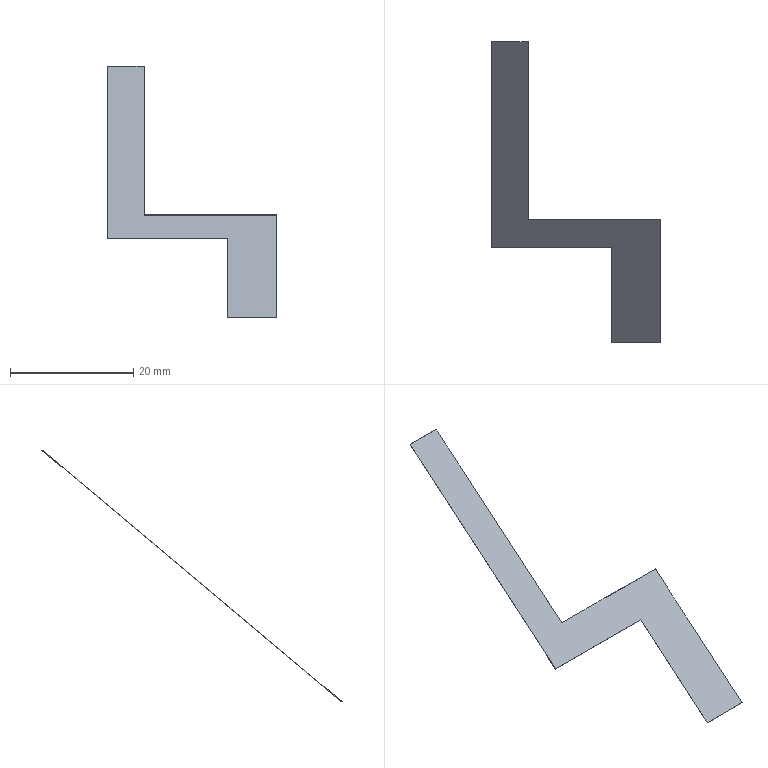Part | SolidWorks | features BaseBody 1 | 1 solid | 10 faces | box 27.548 x 48.792 x 40.953 mm | volume 27.56 mm3 | plane 10
STEP:
#1=CARTESIAN_POINT('',(-790.999,693.76,399.723));
#2=VERTEX_POINT('',#1);
#3=CARTESIAN_POINT('',(-790.999,660.321,371.664));
#4=VERTEX_POINT('',#3);
#5=CARTESIAN_POINT('',(-790.999,693.76,399.723));
#6=DIRECTION('',(0.000001286,-0.766,-0.6428));
#7=VECTOR('',#6,1000.);
#8=LINE('',#5,#7);
#9=EDGE_CURVE('',#2,#4,#8,.T.);
#10=ORIENTED_EDGE('',*,*,#9,.F.);
#11=CARTESIAN_POINT('',(-790.999,693.792,399.685));
#12=VERTEX_POINT('',#11);
#13=CARTESIAN_POINT('',(-790.999,693.792,399.685));
#14=DIRECTION('',(0.000000993,-0.6428,0.766));
#15=VECTOR('',#14,1000.);
#16=LINE('',#13,#15);
#17=EDGE_CURVE('',#12,#2,#16,.T.);
#18=ORIENTED_EDGE('',*,*,#17,.F.);
#19=CARTESIAN_POINT('',(-790.999,660.353,371.626));
#20=VERTEX_POINT('',#19);
#21=CARTESIAN_POINT('',(-790.999,660.353,371.626));
#22=DIRECTION('',(-0.000001286,0.766,0.6428));
#23=VECTOR('',#22,1000.);
#24=LINE('',#21,#23);
#25=EDGE_CURVE('',#20,#12,#24,.T.);
#26=ORIENTED_EDGE('',*,*,#25,.F.);
#27=CARTESIAN_POINT('',(-790.999,660.321,371.664));
#28=DIRECTION('',(-0.000000993,0.6428,-0.766));
#29=VECTOR('',#28,1000.);
#30=LINE('',#27,#29);
#31=EDGE_CURVE('',#4,#20,#30,.T.);
#32=ORIENTED_EDGE('',*,*,#31,.F.);
#33=EDGE_LOOP('',(#10,#18,#26,#32));
#34=FACE_OUTER_BOUND('',#33,.T.);
#35=CARTESIAN_POINT('',(-790.999,679.505,387.696));
#36=DIRECTION('',(1.,0.000001623,0.000000066));
#37=DIRECTION('',(0.000001286,-0.766,-0.6428));
#38=AXIS2_PLACEMENT_3D('',#35,#36,#37);
#39=PLANE('',#38);
#40=ADVANCED_FACE('',(#34),#39,.F.);
#41=CARTESIAN_POINT('',(-771.451,660.353,371.626));
#42=VERTEX_POINT('',#41);
#43=CARTESIAN_POINT('',(-790.999,660.353,371.626));
#44=DIRECTION('',(1.,0.000001623,0.000000066));
#45=VECTOR('',#44,1000.);
#46=LINE('',#43,#45);
#47=EDGE_CURVE('',#20,#42,#46,.T.);
#48=ORIENTED_EDGE('',*,*,#47,.T.);
#49=CARTESIAN_POINT('',(-771.451,660.321,371.664));
#50=VERTEX_POINT('',#49);
#51=CARTESIAN_POINT('',(-771.451,660.321,371.664));
#52=DIRECTION('',(-0.000000993,0.6428,-0.766));
#53=VECTOR('',#52,1000.);
#54=LINE('',#51,#53);
#55=EDGE_CURVE('',#50,#42,#54,.T.);
#56=ORIENTED_EDGE('',*,*,#55,.F.);
#57=CARTESIAN_POINT('',(-790.999,660.321,371.664));
#58=DIRECTION('',(1.,0.000001623,0.000000066));
#59=VECTOR('',#58,1000.);
#60=LINE('',#57,#59);
#61=EDGE_CURVE('',#4,#50,#60,.T.);
#62=ORIENTED_EDGE('',*,*,#61,.F.);
#63=ORIENTED_EDGE('',*,*,#31,.T.);
#64=EDGE_LOOP('',(#48,#56,#62,#63));
#65=FACE_OUTER_BOUND('',#64,.T.);
#66=CARTESIAN_POINT('',(-772.451,660.353,371.626));
#67=DIRECTION('',(-0.000001286,0.766,0.6428));
#68=DIRECTION('',(0.000000993,-0.6428,0.766));
#69=AXIS2_PLACEMENT_3D('',#66,#67,#68);
#70=PLANE('',#69);
#71=ADVANCED_FACE('',(#65),#70,.F.);
#72=CARTESIAN_POINT('',(-771.451,645.,358.809));
#73=VERTEX_POINT('',#72);
#74=CARTESIAN_POINT('',(-771.451,645.,358.809));
#75=DIRECTION('',(-0.000001286,0.766,0.6428));
#76=VECTOR('',#75,1000.);
#77=LINE('',#74,#76);
#78=EDGE_CURVE('',#73,#50,#77,.T.);
#79=ORIENTED_EDGE('',*,*,#78,.F.);
#80=CARTESIAN_POINT('',(-763.451,645.,358.809));
#81=VERTEX_POINT('',#80);
#82=CARTESIAN_POINT('',(-763.451,645.,358.809));
#83=DIRECTION('',(-1.,-0.000001623,-0.000000066));
#84=VECTOR('',#83,1000.);
#85=LINE('',#82,#84);
#86=EDGE_CURVE('',#81,#73,#85,.T.);
#87=ORIENTED_EDGE('',*,*,#86,.F.);
#88=CARTESIAN_POINT('',(-763.451,664.918,375.521));
#89=VERTEX_POINT('',#88);
#90=CARTESIAN_POINT('',(-763.451,664.918,375.521));
#91=DIRECTION('',(0.000001286,-0.766,-0.6428));
#92=VECTOR('',#91,1000.);
#93=LINE('',#90,#92);
#94=EDGE_CURVE('',#89,#81,#93,.T.);
#95=ORIENTED_EDGE('',*,*,#94,.F.);
#96=CARTESIAN_POINT('',(-784.999,664.918,375.521));
#97=VERTEX_POINT('',#96);
#98=CARTESIAN_POINT('',(-784.999,664.918,375.521));
#99=DIRECTION('',(1.,0.000001623,0.000000066));
#100=VECTOR('',#99,1000.);
#101=LINE('',#98,#100);
#102=EDGE_CURVE('',#97,#89,#101,.T.);
#103=ORIENTED_EDGE('',*,*,#102,.F.);
#104=CARTESIAN_POINT('',(-784.999,693.76,399.723));
#105=VERTEX_POINT('',#104);
#106=CARTESIAN_POINT('',(-784.999,693.76,399.723));
#107=DIRECTION('',(0.000001286,-0.766,-0.6428));
#108=VECTOR('',#107,1000.);
#109=LINE('',#106,#108);
#110=EDGE_CURVE('',#105,#97,#109,.T.);
#111=ORIENTED_EDGE('',*,*,#110,.F.);
#112=CARTESIAN_POINT('',(-790.999,693.76,399.723));
#113=DIRECTION('',(1.,0.000001623,0.000000066));
#114=VECTOR('',#113,1000.);
#115=LINE('',#112,#114);
#116=EDGE_CURVE('',#2,#105,#115,.T.);
#117=ORIENTED_EDGE('',*,*,#116,.F.);
#118=ORIENTED_EDGE('',*,*,#9,.T.);
#119=ORIENTED_EDGE('',*,*,#61,.T.);
#120=EDGE_LOOP('',(#79,#87,#95,#103,#111,#117,#118,#119));
#121=FACE_OUTER_BOUND('',#120,.T.);
#122=CARTESIAN_POINT('',(-733.13,689.185,395.884));
#123=DIRECTION('',(-0.000000993,0.6428,-0.766));
#124=DIRECTION('',(1.,0.000001623,0.000000066));
#125=AXIS2_PLACEMENT_3D('',#122,#123,#124);
#126=PLANE('',#125);
#127=ADVANCED_FACE('',(#121),#126,.F.);
#128=CARTESIAN_POINT('',(-784.999,693.792,399.685));
#129=VERTEX_POINT('',#128);
#130=CARTESIAN_POINT('',(-784.999,693.792,399.685));
#131=DIRECTION('',(-1.,-0.000001623,-0.000000066));
#132=VECTOR('',#131,1000.);
#133=LINE('',#130,#132);
#134=EDGE_CURVE('',#129,#12,#133,.T.);
#135=ORIENTED_EDGE('',*,*,#134,.T.);
#136=ORIENTED_EDGE('',*,*,#17,.T.);
#137=ORIENTED_EDGE('',*,*,#116,.T.);
#138=CARTESIAN_POINT('',(-784.999,693.792,399.685));
#139=DIRECTION('',(0.000000993,-0.6428,0.766));
#140=VECTOR('',#139,1000.);
#141=LINE('',#138,#140);
#142=EDGE_CURVE('',#129,#105,#141,.T.);
#143=ORIENTED_EDGE('',*,*,#142,.F.);
#144=EDGE_LOOP('',(#135,#136,#137,#143));
#145=FACE_OUTER_BOUND('',#144,.T.);
#146=CARTESIAN_POINT('',(-799.999,693.792,399.685));
#147=DIRECTION('',(0.000001286,-0.766,-0.6428));
#148=DIRECTION('',(-0.000000993,0.6428,-0.766));
#149=AXIS2_PLACEMENT_3D('',#146,#147,#148);
#150=PLANE('',#149);
#151=ADVANCED_FACE('',(#145),#150,.F.);
#152=CARTESIAN_POINT('',(-784.999,664.95,375.483));
#153=VERTEX_POINT('',#152);
#154=CARTESIAN_POINT('',(-784.999,664.95,375.483));
#155=DIRECTION('',(-0.000001286,0.766,0.6428));
#156=VECTOR('',#155,1000.);
#157=LINE('',#154,#156);
#158=EDGE_CURVE('',#153,#129,#157,.T.);
#159=ORIENTED_EDGE('',*,*,#158,.T.);
#160=ORIENTED_EDGE('',*,*,#142,.T.);
#161=ORIENTED_EDGE('',*,*,#110,.T.);
#162=CARTESIAN_POINT('',(-784.999,664.95,375.483));
#163=DIRECTION('',(0.000000993,-0.6428,0.766));
#164=VECTOR('',#163,1000.);
#165=LINE('',#162,#164);
#166=EDGE_CURVE('',#153,#97,#165,.T.);
#167=ORIENTED_EDGE('',*,*,#166,.F.);
#168=EDGE_LOOP('',(#159,#160,#161,#167));
#169=FACE_OUTER_BOUND('',#168,.T.);
#170=CARTESIAN_POINT('',(-784.999,697.623,402.899));
#171=DIRECTION('',(-1.,-0.000001623,-0.000000066));
#172=DIRECTION('',(-0.000001286,0.766,0.6428));
#173=AXIS2_PLACEMENT_3D('',#170,#171,#172);
#174=PLANE('',#173);
#175=ADVANCED_FACE('',(#169),#174,.F.);
#176=CARTESIAN_POINT('',(-763.451,664.95,375.483));
#177=VERTEX_POINT('',#176);
#178=CARTESIAN_POINT('',(-763.451,664.95,375.483));
#179=DIRECTION('',(-1.,-0.000001623,-0.000000066));
#180=VECTOR('',#179,1000.);
#181=LINE('',#178,#180);
#182=EDGE_CURVE('',#177,#153,#181,.T.);
#183=ORIENTED_EDGE('',*,*,#182,.T.);
#184=ORIENTED_EDGE('',*,*,#166,.T.);
#185=ORIENTED_EDGE('',*,*,#102,.T.);
#186=CARTESIAN_POINT('',(-763.451,664.95,375.483));
#187=DIRECTION('',(0.000000993,-0.6428,0.766));
#188=VECTOR('',#187,1000.);
#189=LINE('',#186,#188);
#190=EDGE_CURVE('',#177,#89,#189,.T.);
#191=ORIENTED_EDGE('',*,*,#190,.F.);
#192=EDGE_LOOP('',(#183,#184,#185,#191));
#193=FACE_OUTER_BOUND('',#192,.T.);
#194=CARTESIAN_POINT('',(-793.999,664.95,375.483));
#195=DIRECTION('',(0.000001286,-0.766,-0.6428));
#196=DIRECTION('',(-1.,-0.000001623,-0.000000066));
#197=AXIS2_PLACEMENT_3D('',#194,#195,#196);
#198=PLANE('',#197);
#199=ADVANCED_FACE('',(#193),#198,.F.);
#200=ORIENTED_EDGE('',*,*,#94,.T.);
#201=CARTESIAN_POINT('',(-763.451,645.033,358.77));
#202=VERTEX_POINT('',#201);
#203=CARTESIAN_POINT('',(-763.451,645.033,358.77));
#204=DIRECTION('',(0.000000993,-0.6428,0.766));
#205=VECTOR('',#204,1000.);
#206=LINE('',#203,#205);
#207=EDGE_CURVE('',#202,#81,#206,.T.);
#208=ORIENTED_EDGE('',*,*,#207,.F.);
#209=CARTESIAN_POINT('',(-763.451,645.033,358.77));
#210=DIRECTION('',(-0.000001286,0.766,0.6428));
#211=VECTOR('',#210,1000.);
#212=LINE('',#209,#211);
#213=EDGE_CURVE('',#202,#177,#212,.T.);
#214=ORIENTED_EDGE('',*,*,#213,.T.);
#215=ORIENTED_EDGE('',*,*,#190,.T.);
#216=EDGE_LOOP('',(#200,#208,#214,#215));
#217=FACE_OUTER_BOUND('',#216,.T.);
#218=CARTESIAN_POINT('',(-763.451,684.101,391.552));
#219=DIRECTION('',(-1.,-0.000001623,-0.000000066));
#220=DIRECTION('',(-0.000001286,0.766,0.6428));
#221=AXIS2_PLACEMENT_3D('',#218,#219,#220);
#222=PLANE('',#221);
#223=ADVANCED_FACE('',(#217),#222,.F.);
#224=ORIENTED_EDGE('',*,*,#134,.F.);
#225=ORIENTED_EDGE('',*,*,#158,.F.);
#226=ORIENTED_EDGE('',*,*,#182,.F.);
#227=ORIENTED_EDGE('',*,*,#213,.F.);
#228=CARTESIAN_POINT('',(-771.451,645.033,358.77));
#229=VERTEX_POINT('',#228);
#230=CARTESIAN_POINT('',(-771.451,645.033,358.77));
#231=DIRECTION('',(1.,0.000001623,0.000000066));
#232=VECTOR('',#231,1000.);
#233=LINE('',#230,#232);
#234=EDGE_CURVE('',#229,#202,#233,.T.);
#235=ORIENTED_EDGE('',*,*,#234,.F.);
#236=CARTESIAN_POINT('',(-771.451,660.353,371.626));
#237=DIRECTION('',(0.000001286,-0.766,-0.6428));
#238=VECTOR('',#237,1000.);
#239=LINE('',#236,#238);
#240=EDGE_CURVE('',#42,#229,#239,.T.);
#241=ORIENTED_EDGE('',*,*,#240,.F.);
#242=ORIENTED_EDGE('',*,*,#47,.F.);
#243=ORIENTED_EDGE('',*,*,#25,.T.);
#244=EDGE_LOOP('',(#224,#225,#226,#227,#235,#241,#242,#243));
#245=FACE_OUTER_BOUND('',#244,.T.);
#246=CARTESIAN_POINT('',(-733.13,689.217,395.846));
#247=DIRECTION('',(-0.000000993,0.6428,-0.766));
#248=DIRECTION('',(1.,0.000001623,0.000000066));
#249=AXIS2_PLACEMENT_3D('',#246,#247,#248);
#250=PLANE('',#249);
#251=ADVANCED_FACE('',(#245),#250,.T.);
#252=ORIENTED_EDGE('',*,*,#240,.T.);
#253=CARTESIAN_POINT('',(-771.451,645.033,358.77));
#254=DIRECTION('',(0.000000993,-0.6428,0.766));
#255=VECTOR('',#254,1000.);
#256=LINE('',#253,#255);
#257=EDGE_CURVE('',#229,#73,#256,.T.);
#258=ORIENTED_EDGE('',*,*,#257,.T.);
#259=ORIENTED_EDGE('',*,*,#78,.T.);
#260=ORIENTED_EDGE('',*,*,#55,.T.);
#261=EDGE_LOOP('',(#252,#258,#259,#260));
#262=FACE_OUTER_BOUND('',#261,.T.);
#263=CARTESIAN_POINT('',(-771.451,656.523,368.412));
#264=DIRECTION('',(1.,0.000001623,0.000000066));
#265=DIRECTION('',(0.000001286,-0.766,-0.6428));
#266=AXIS2_PLACEMENT_3D('',#263,#264,#265);
#267=PLANE('',#266);
#268=ADVANCED_FACE('',(#262),#267,.F.);
#269=ORIENTED_EDGE('',*,*,#234,.T.);
#270=ORIENTED_EDGE('',*,*,#207,.T.);
#271=ORIENTED_EDGE('',*,*,#86,.T.);
#272=ORIENTED_EDGE('',*,*,#257,.F.);
#273=EDGE_LOOP('',(#269,#270,#271,#272));
#274=FACE_OUTER_BOUND('',#273,.T.);
#275=CARTESIAN_POINT('',(-760.451,645.033,358.77));
#276=DIRECTION('',(-0.000001286,0.766,0.6428));
#277=DIRECTION('',(1.,0.000001623,0.000000066));
#278=AXIS2_PLACEMENT_3D('',#275,#276,#277);
#279=PLANE('',#278);
#280=ADVANCED_FACE('',(#274),#279,.F.);
#281=CLOSED_SHELL('',(#40,#71,#127,#151,#175,#199,#223,#251,#268,#280));
#282=MANIFOLD_SOLID_BREP('',#281);
#283=CARTESIAN_POINT('',(0.,0.,0.));
#284=DIRECTION('',(0.,0.,1.));
#285=DIRECTION('',(1.,0.,0.));
#286=AXIS2_PLACEMENT_3D('',#283,#284,#285);
#287=(LENGTH_UNIT()NAMED_UNIT(*)SI_UNIT(.MILLI.,.METRE.));
#288=UNCERTAINTY_MEASURE_WITH_UNIT(LENGTH_MEASURE(0.00001),#287,'','');
#289=(NAMED_UNIT(*)PLANE_ANGLE_UNIT()SI_UNIT($,.RADIAN.));
#290=(NAMED_UNIT(*)SI_UNIT($,.STERADIAN.)SOLID_ANGLE_UNIT());
#291=(GEOMETRIC_REPRESENTATION_CONTEXT(3)GLOBAL_UNCERTAINTY_ASSIGNED_CONTEXT((#288))GLOBAL_UNIT_ASSIGNED_CONTEXT((#287,#289,#290))REPRESENTATION_CONTEXT('',''));
#292=ADVANCED_BREP_SHAPE_REPRESENTATION('',(#282,#286),#291);